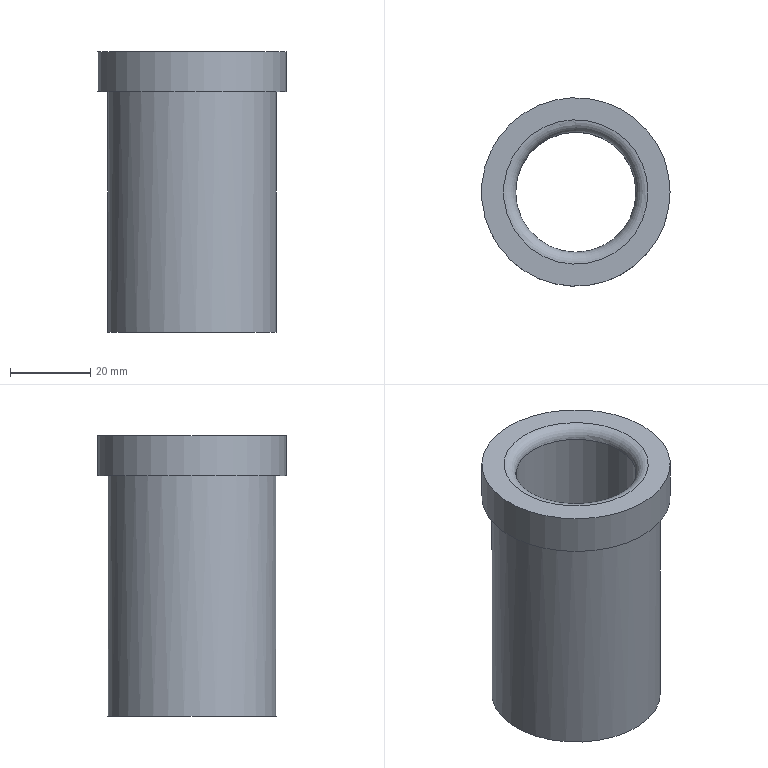Part | NX | features MPPJ 2 | 1 solid | 8 faces | box 47 x 47 x 70 mm | volume 50616 mm3 | plane 3 | cylinder 3 | torus 2 | commonest cylinder face diameters 30 x1 42 x1 47 x1
STEP:
#1=CARTESIAN_POINT('',(124.,142.,0.5));
#2=VERTEX_POINT('',#1);
#3=CARTESIAN_POINT('',(142.,142.,0.5));
#4=DIRECTION('',(0.,0.,-1.));
#5=DIRECTION('',(-1.,0.,0.));
#6=AXIS2_PLACEMENT_3D('',#3,#4,#5);
#7=CIRCLE('',#6,18.);
#8=EDGE_CURVE('',#2,#2,#7,.F.);
#9=ORIENTED_EDGE('',*,*,#8,.T.);
#10=EDGE_LOOP('',(#9));
#11=FACE_BOUND('',#10,.T.);
#12=CARTESIAN_POINT('',(163.,142.,0.5));
#13=VERTEX_POINT('',#12);
#14=CARTESIAN_POINT('',(142.,142.,0.5));
#15=DIRECTION('',(0.,0.,1.));
#16=DIRECTION('',(1.,0.,0.));
#17=AXIS2_PLACEMENT_3D('',#14,#15,#16);
#18=CIRCLE('',#17,21.);
#19=EDGE_CURVE('',#13,#13,#18,.T.);
#20=ORIENTED_EDGE('',*,*,#19,.F.);
#21=EDGE_LOOP('',(#20));
#22=FACE_BOUND('',#21,.T.);
#23=CARTESIAN_POINT('',(142.,142.,0.5));
#24=DIRECTION('',(0.,0.,-1.));
#25=DIRECTION('',(-1.,0.,0.));
#26=AXIS2_PLACEMENT_3D('',#23,#24,#25);
#27=PLANE('',#26);
#28=ADVANCED_FACE('',(#11,#22),#27,.T.);
#29=CARTESIAN_POINT('',(160.,142.,70.5));
#30=VERTEX_POINT('',#29);
#31=CARTESIAN_POINT('',(142.,142.,70.5));
#32=DIRECTION('',(0.,0.,1.));
#33=DIRECTION('',(1.,0.,0.));
#34=AXIS2_PLACEMENT_3D('',#31,#32,#33);
#35=CIRCLE('',#34,18.);
#36=EDGE_CURVE('',#30,#30,#35,.F.);
#37=ORIENTED_EDGE('',*,*,#36,.T.);
#38=EDGE_LOOP('',(#37));
#39=FACE_BOUND('',#38,.T.);
#40=CARTESIAN_POINT('',(165.5,142.,70.5));
#41=VERTEX_POINT('',#40);
#42=CARTESIAN_POINT('',(142.,142.,70.5));
#43=DIRECTION('',(0.,0.,-1.));
#44=DIRECTION('',(1.,0.,0.));
#45=AXIS2_PLACEMENT_3D('',#42,#43,#44);
#46=CIRCLE('',#45,23.5);
#47=EDGE_CURVE('',#41,#41,#46,.T.);
#48=ORIENTED_EDGE('',*,*,#47,.F.);
#49=EDGE_LOOP('',(#48));
#50=FACE_BOUND('',#49,.T.);
#51=CARTESIAN_POINT('',(142.,142.,70.5));
#52=DIRECTION('',(0.,0.,1.));
#53=DIRECTION('',(1.,0.,0.));
#54=AXIS2_PLACEMENT_3D('',#51,#52,#53);
#55=PLANE('',#54);
#56=ADVANCED_FACE('',(#39,#50),#55,.T.);
#57=CARTESIAN_POINT('',(121.,142.,60.5));
#58=VERTEX_POINT('',#57);
#59=CARTESIAN_POINT('',(142.,142.,60.5));
#60=DIRECTION('',(0.,0.,-1.));
#61=DIRECTION('',(-1.,0.,0.));
#62=AXIS2_PLACEMENT_3D('',#59,#60,#61);
#63=CIRCLE('',#62,21.);
#64=EDGE_CURVE('',#58,#58,#63,.F.);
#65=ORIENTED_EDGE('',*,*,#64,.F.);
#66=EDGE_LOOP('',(#65));
#67=FACE_BOUND('',#66,.T.);
#68=ORIENTED_EDGE('',*,*,#19,.T.);
#69=EDGE_LOOP('',(#68));
#70=FACE_BOUND('',#69,.T.);
#71=CARTESIAN_POINT('',(142.,142.,70.5));
#72=DIRECTION('',(0.,0.,-1.));
#73=DIRECTION('',(1.,0.,0.));
#74=AXIS2_PLACEMENT_3D('',#71,#72,#73);
#75=CYLINDRICAL_SURFACE('',#74,21.);
#76=ADVANCED_FACE('',(#67,#70),#75,.T.);
#77=ORIENTED_EDGE('',*,*,#64,.T.);
#78=EDGE_LOOP('',(#77));
#79=FACE_BOUND('',#78,.T.);
#80=CARTESIAN_POINT('',(165.5,142.,60.5));
#81=VERTEX_POINT('',#80);
#82=CARTESIAN_POINT('',(142.,142.,60.5));
#83=DIRECTION('',(0.,0.,1.));
#84=DIRECTION('',(1.,0.,0.));
#85=AXIS2_PLACEMENT_3D('',#82,#83,#84);
#86=CIRCLE('',#85,23.5);
#87=EDGE_CURVE('',#81,#81,#86,.T.);
#88=ORIENTED_EDGE('',*,*,#87,.F.);
#89=EDGE_LOOP('',(#88));
#90=FACE_BOUND('',#89,.T.);
#91=CARTESIAN_POINT('',(142.,142.,60.5));
#92=DIRECTION('',(0.,0.,-1.));
#93=DIRECTION('',(-1.,0.,0.));
#94=AXIS2_PLACEMENT_3D('',#91,#92,#93);
#95=PLANE('',#94);
#96=ADVANCED_FACE('',(#79,#90),#95,.T.);
#97=ORIENTED_EDGE('',*,*,#87,.T.);
#98=EDGE_LOOP('',(#97));
#99=FACE_BOUND('',#98,.T.);
#100=ORIENTED_EDGE('',*,*,#47,.T.);
#101=EDGE_LOOP('',(#100));
#102=FACE_BOUND('',#101,.T.);
#103=CARTESIAN_POINT('',(142.,142.,70.5));
#104=DIRECTION('',(0.,0.,-1.));
#105=DIRECTION('',(1.,0.,0.));
#106=AXIS2_PLACEMENT_3D('',#103,#104,#105);
#107=CYLINDRICAL_SURFACE('',#106,23.5);
#108=ADVANCED_FACE('',(#99,#102),#107,.T.);
#109=CARTESIAN_POINT('',(157.,142.,67.5));
#110=VERTEX_POINT('',#109);
#111=CARTESIAN_POINT('',(142.,142.,67.5));
#112=DIRECTION('',(0.,0.,1.));
#113=DIRECTION('',(1.,0.,0.));
#114=AXIS2_PLACEMENT_3D('',#111,#112,#113);
#115=CIRCLE('',#114,15.);
#116=EDGE_CURVE('',#110,#110,#115,.T.);
#117=ORIENTED_EDGE('',*,*,#116,.T.);
#118=EDGE_LOOP('',(#117));
#119=FACE_BOUND('',#118,.T.);
#120=CARTESIAN_POINT('',(127.,142.,3.5));
#121=VERTEX_POINT('',#120);
#122=CARTESIAN_POINT('',(142.,142.,3.5));
#123=DIRECTION('',(0.,0.,-1.));
#124=DIRECTION('',(-1.,0.,0.));
#125=AXIS2_PLACEMENT_3D('',#122,#123,#124);
#126=CIRCLE('',#125,15.);
#127=EDGE_CURVE('',#121,#121,#126,.T.);
#128=ORIENTED_EDGE('',*,*,#127,.T.);
#129=EDGE_LOOP('',(#128));
#130=FACE_BOUND('',#129,.T.);
#131=CARTESIAN_POINT('',(142.,142.,70.5));
#132=DIRECTION('',(0.,0.,-1.));
#133=DIRECTION('',(1.,0.,0.));
#134=AXIS2_PLACEMENT_3D('',#131,#132,#133);
#135=CYLINDRICAL_SURFACE('',#134,15.);
#136=ADVANCED_FACE('',(#119,#130),#135,.F.);
#137=ORIENTED_EDGE('',*,*,#116,.F.);
#138=EDGE_LOOP('',(#137));
#139=FACE_BOUND('',#138,.T.);
#140=ORIENTED_EDGE('',*,*,#36,.F.);
#141=EDGE_LOOP('',(#140));
#142=FACE_BOUND('',#141,.T.);
#143=CARTESIAN_POINT('',(142.,142.,67.5));
#144=DIRECTION('',(0.,0.,1.));
#145=DIRECTION('',(1.,0.,0.));
#146=AXIS2_PLACEMENT_3D('',#143,#144,#145);
#147=TOROIDAL_SURFACE('',#146,18.,3.);
#148=ADVANCED_FACE('',(#139,#142),#147,.T.);
#149=ORIENTED_EDGE('',*,*,#127,.F.);
#150=EDGE_LOOP('',(#149));
#151=FACE_BOUND('',#150,.T.);
#152=ORIENTED_EDGE('',*,*,#8,.F.);
#153=EDGE_LOOP('',(#152));
#154=FACE_BOUND('',#153,.T.);
#155=CARTESIAN_POINT('',(142.,142.,3.5));
#156=DIRECTION('',(0.,0.,-1.));
#157=DIRECTION('',(-1.,0.,0.));
#158=AXIS2_PLACEMENT_3D('',#155,#156,#157);
#159=TOROIDAL_SURFACE('',#158,18.,3.);
#160=ADVANCED_FACE('',(#151,#154),#159,.T.);
#161=CLOSED_SHELL('',(#28,#56,#76,#96,#108,#136,#148,#160));
#162=MANIFOLD_SOLID_BREP('',#161);
#163=(LENGTH_UNIT()NAMED_UNIT(*)SI_UNIT(.MILLI.,.METRE.));
#164=UNCERTAINTY_MEASURE_WITH_UNIT(LENGTH_MEASURE(0.00001),#163,'','');
#165=(NAMED_UNIT(*)PLANE_ANGLE_UNIT()SI_UNIT($,.RADIAN.));
#166=(NAMED_UNIT(*)SI_UNIT($,.STERADIAN.)SOLID_ANGLE_UNIT());
#167=(GEOMETRIC_REPRESENTATION_CONTEXT(3)GLOBAL_UNCERTAINTY_ASSIGNED_CONTEXT((#164))GLOBAL_UNIT_ASSIGNED_CONTEXT((#163,#165,#166))REPRESENTATION_CONTEXT('',''));
#168=ADVANCED_BREP_SHAPE_REPRESENTATION('',(#162),#167);